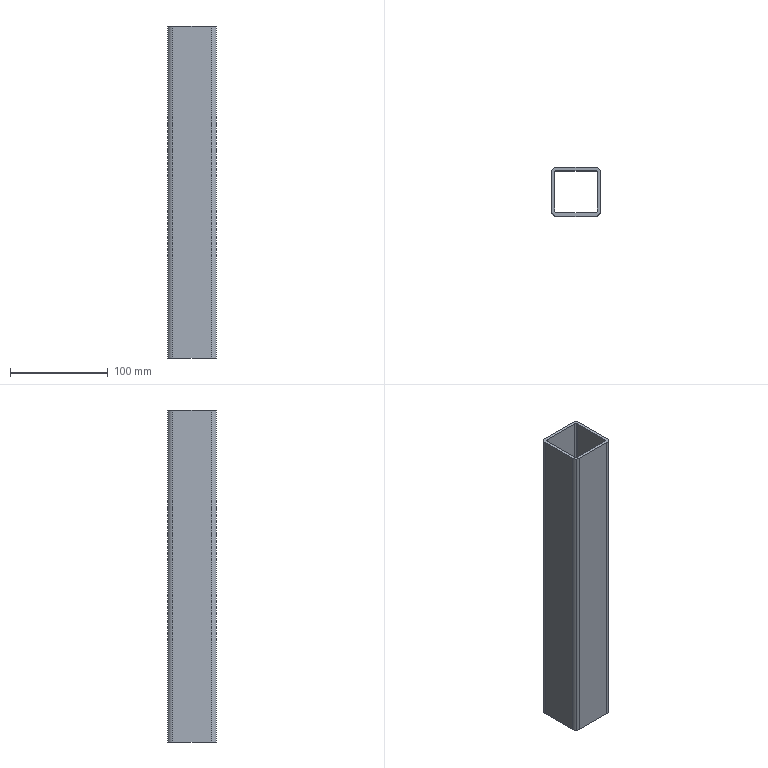Part | STEP file | POST.SQ.PIPE.4.stp | 1 solid | 26 faces | box 50 x 50 x 340 mm | volume 196949 mm3 | cylinder 16 | plane 10 | commonest cylinder face diameters 4 x8 10.4 x8